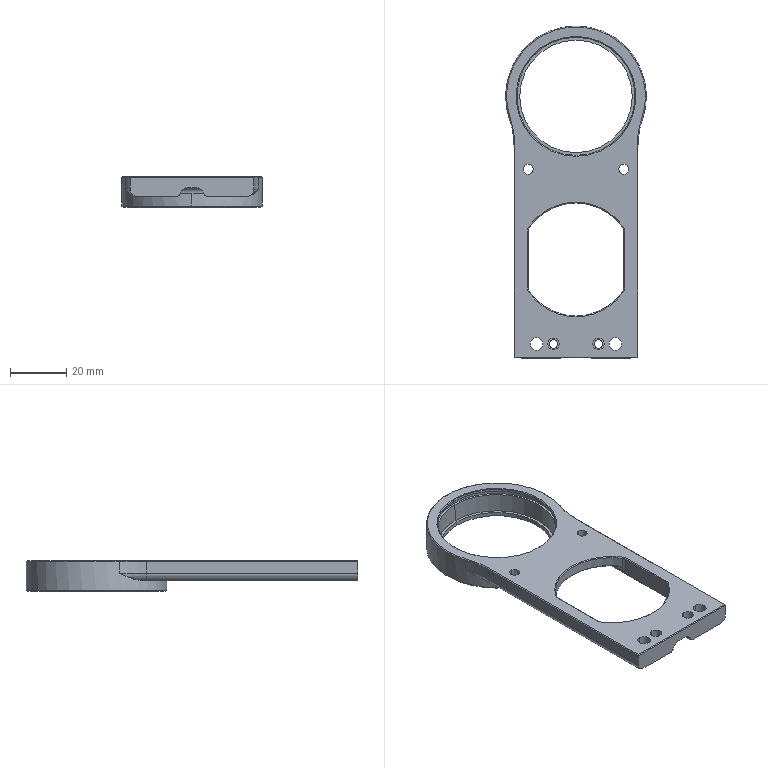Part | 1 solid | 144 faces | box 50 x 118 x 11 mm | volume 16974 mm3 | cylinder 61 | plane 33 | cone 29 | spline 10 | torus 7 | sphere 4 | commonest cylinder face diameters 4 x20 3 x4 3.5 x4 4.5 x4 7 x4 40.2 x3